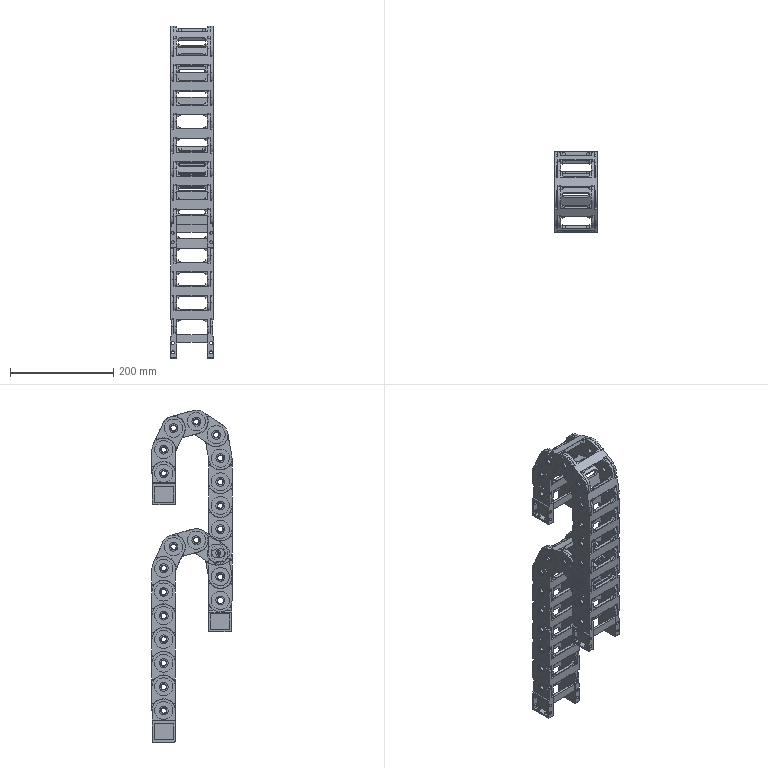Part | SolidWorks | features BaseBody 14, LPattern 4 | 24 solids | 6042 faces | volume 1173984 mm3 | cylinder 3778 | plane 2264 | commonest cylinder face diameters 2 x632 1 x420 4 x270 20.12 x230 41.64 x210 17.1 x184